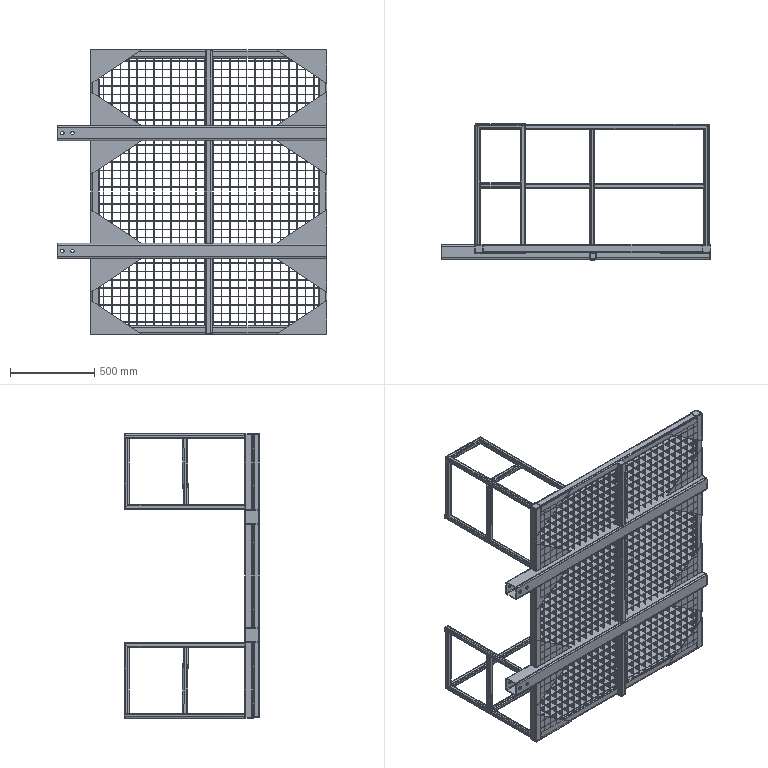Part | STEP file | REAR_RECEIVING_PLATFORMV11_Default<Machined> | 155 solids | 1314 faces | box 1600 x 805 x 1690 mm | volume 26046895 mm3 | plane 1034 | cylinder 280 | commonest cylinder face diameters 8 x132 16 x108 20 x24 10 x16